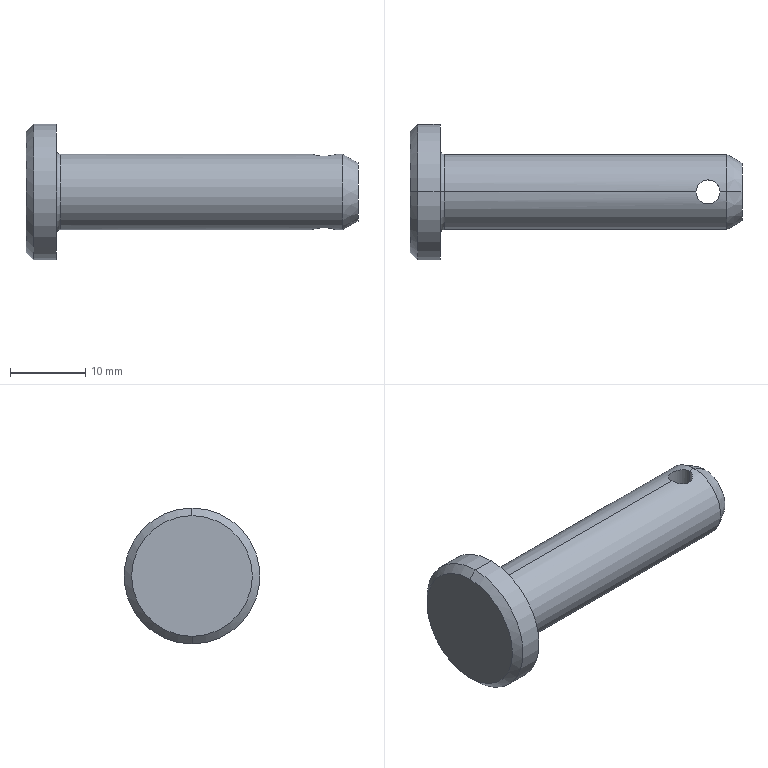Part | SolidWorks | features Chamfer 1, Fillet 1, ICE 1, Revolution 1 | 1 solid | 15 faces | box 44 x 18 x 18 mm | volume 4022 mm3 | cylinder 6 | cone 4 | plane 3 | torus 2 | commonest cylinder face diameters 3.2 x2 10 x2 18 x2
STEP:
#1=CARTESIAN_POINT('',(44.,0.,-3.845));
#2=VERTEX_POINT('',#1);
#3=CARTESIAN_POINT('',(44.,0.,3.845));
#4=VERTEX_POINT('',#3);
#5=CARTESIAN_POINT('',(44.,0.,0.));
#6=DIRECTION('',(1.,0.,0.));
#7=DIRECTION('',(0.,0.,-1.));
#8=AXIS2_PLACEMENT_3D('',#5,#6,#7);
#9=CIRCLE('',#8,3.845);
#10=EDGE_CURVE('',#2,#4,#9,.T.);
#11=ORIENTED_EDGE('',*,*,#10,.F.);
#12=CARTESIAN_POINT('',(42.,0.,-5.));
#13=VERTEX_POINT('',#12);
#14=CARTESIAN_POINT('',(44.,0.,-3.845));
#15=DIRECTION('',(-0.866,0.,-0.5));
#16=VECTOR('',#15,1000.);
#17=LINE('',#14,#16);
#18=EDGE_CURVE('',#2,#13,#17,.T.);
#19=ORIENTED_EDGE('',*,*,#18,.T.);
#20=CARTESIAN_POINT('',(42.,0.,5.));
#21=VERTEX_POINT('',#20);
#22=CARTESIAN_POINT('',(42.,0.,0.));
#23=DIRECTION('',(-1.,0.,0.));
#24=DIRECTION('',(0.,0.,-1.));
#25=AXIS2_PLACEMENT_3D('',#22,#23,#24);
#26=CIRCLE('',#25,5.);
#27=EDGE_CURVE('',#21,#13,#26,.T.);
#28=ORIENTED_EDGE('',*,*,#27,.F.);
#29=CARTESIAN_POINT('',(44.,0.,3.845));
#30=DIRECTION('',(-0.866,0.,0.5));
#31=VECTOR('',#30,1000.);
#32=LINE('',#29,#31);
#33=EDGE_CURVE('',#4,#21,#32,.T.);
#34=ORIENTED_EDGE('',*,*,#33,.F.);
#35=EDGE_LOOP('',(#11,#19,#28,#34));
#36=FACE_OUTER_BOUND('',#35,.T.);
#37=CARTESIAN_POINT('',(44.,0.,0.));
#38=DIRECTION('',(-1.,0.,0.));
#39=DIRECTION('',(0.,0.,1.));
#40=AXIS2_PLACEMENT_3D('',#37,#38,#39);
#41=CONICAL_SURFACE('',#40,3.845,0.5236);
#42=ADVANCED_FACE('',(#36),#41,.T.);
#43=CARTESIAN_POINT('',(4.6,0.,5.));
#44=VERTEX_POINT('',#43);
#45=CARTESIAN_POINT('',(4.6,0.,-5.));
#46=VERTEX_POINT('',#45);
#47=CARTESIAN_POINT('',(4.6,0.,0.));
#48=DIRECTION('',(1.,0.,0.));
#49=DIRECTION('',(0.,0.,-1.));
#50=AXIS2_PLACEMENT_3D('',#47,#48,#49);
#51=CIRCLE('',#50,5.);
#52=EDGE_CURVE('',#44,#46,#51,.T.);
#53=ORIENTED_EDGE('',*,*,#52,.F.);
#54=CARTESIAN_POINT('',(4.,0.,5.6));
#55=VERTEX_POINT('',#54);
#56=CARTESIAN_POINT('',(4.6,0.,5.6));
#57=DIRECTION('',(0.,1.,0.));
#58=DIRECTION('',(0.,0.,1.));
#59=AXIS2_PLACEMENT_3D('',#56,#57,#58);
#60=CIRCLE('',#59,0.6);
#61=EDGE_CURVE('',#44,#55,#60,.T.);
#62=ORIENTED_EDGE('',*,*,#61,.T.);
#63=CARTESIAN_POINT('',(4.,0.,-5.6));
#64=VERTEX_POINT('',#63);
#65=CARTESIAN_POINT('',(4.,0.,0.));
#66=DIRECTION('',(-1.,0.,0.));
#67=DIRECTION('',(0.,0.,-1.));
#68=AXIS2_PLACEMENT_3D('',#65,#66,#67);
#69=CIRCLE('',#68,5.6);
#70=EDGE_CURVE('',#64,#55,#69,.T.);
#71=ORIENTED_EDGE('',*,*,#70,.F.);
#72=CARTESIAN_POINT('',(4.6,0.,-5.6));
#73=DIRECTION('',(0.,-1.,0.));
#74=DIRECTION('',(0.,0.,-1.));
#75=AXIS2_PLACEMENT_3D('',#72,#73,#74);
#76=CIRCLE('',#75,0.6);
#77=EDGE_CURVE('',#46,#64,#76,.T.);
#78=ORIENTED_EDGE('',*,*,#77,.F.);
#79=EDGE_LOOP('',(#53,#62,#71,#78));
#80=FACE_OUTER_BOUND('',#79,.T.);
#81=CARTESIAN_POINT('',(4.6,0.,0.));
#82=DIRECTION('',(1.,0.,0.));
#83=DIRECTION('',(0.,0.,-1.));
#84=AXIS2_PLACEMENT_3D('',#81,#82,#83);
#85=TOROIDAL_SURFACE('',#84,5.6,0.6);
#86=ADVANCED_FACE('',(#80),#85,.F.);
#87=CARTESIAN_POINT('',(41.1,0.,-5.));
#88=VERTEX_POINT('',#87);
#89=CARTESIAN_POINT('',(37.9,0.,-5.));
#90=VERTEX_POINT('',#89);
#91=CARTESIAN_POINT('',(41.1,0.,-5.));
#92=CARTESIAN_POINT('',(41.1,-0.2097,-5.));
#93=CARTESIAN_POINT('',(41.058,-0.4215,-4.986));
#94=CARTESIAN_POINT('',(40.937,-0.711,-4.95));
#95=CARTESIAN_POINT('',(40.887,-0.8046,-4.936));
#96=CARTESIAN_POINT('',(40.771,-0.9775,-4.904));
#97=CARTESIAN_POINT('',(40.705,-1.058,-4.887));
#98=CARTESIAN_POINT('',(40.484,-1.279,-4.836));
#99=CARTESIAN_POINT('',(40.309,-1.396,-4.802));
#100=CARTESIAN_POINT('',(40.017,-1.518,-4.764));
#101=CARTESIAN_POINT('',(39.917,-1.548,-4.754));
#102=CARTESIAN_POINT('',(39.712,-1.589,-4.741));
#103=CARTESIAN_POINT('',(39.605,-1.6,-4.737));
#104=CARTESIAN_POINT('',(39.395,-1.6,-4.737));
#105=CARTESIAN_POINT('',(39.29,-1.59,-4.741));
#106=CARTESIAN_POINT('',(39.084,-1.548,-4.754));
#107=CARTESIAN_POINT('',(38.982,-1.517,-4.764));
#108=CARTESIAN_POINT('',(38.693,-1.397,-4.802));
#109=CARTESIAN_POINT('',(38.516,-1.278,-4.836));
#110=CARTESIAN_POINT('',(38.296,-1.058,-4.887));
#111=CARTESIAN_POINT('',(38.228,-0.9767,-4.904));
#112=CARTESIAN_POINT('',(38.113,-0.8036,-4.936));
#113=CARTESIAN_POINT('',(38.063,-0.7121,-4.95));
#114=CARTESIAN_POINT('',(37.983,-0.5188,-4.974));
#115=CARTESIAN_POINT('',(37.952,-0.4167,-4.984));
#116=CARTESIAN_POINT('',(37.911,-0.2111,-4.997));
#117=CARTESIAN_POINT('',(37.9,-0.1064,-5.));
#118=CARTESIAN_POINT('',(37.9,0.,-5.));
#119=B_SPLINE_CURVE_WITH_KNOTS('',3,(#91,#92,#93,#94,#95,#96,#97,#98,#99,#100,#101,#102,#103,#104,#105,#106,#107,#108,#109,#110,#111,#112,#113,#114,#115,#116,#117,#118),.UNSPECIFIED.,.F.,.F.,(4,2,2,2,2,2,2,2,2,2,2,2,2,4),(0.005036,0.005665,0.00598,0.006294,0.006924,0.007238,0.007553,0.007867,0.008182,0.008811,0.009126,0.009441,0.009755,0.01007),.UNSPECIFIED.);
#120=EDGE_CURVE('',#88,#90,#119,.T.);
#121=ORIENTED_EDGE('',*,*,#120,.T.);
#122=CARTESIAN_POINT('',(37.9,0.,5.));
#123=VERTEX_POINT('',#122);
#124=CARTESIAN_POINT('',(37.9,0.,-9.));
#125=DIRECTION('',(0.,0.,1.));
#126=VECTOR('',#125,1000.);
#127=LINE('',#124,#126);
#128=EDGE_CURVE('',#90,#123,#127,.T.);
#129=ORIENTED_EDGE('',*,*,#128,.T.);
#130=CARTESIAN_POINT('',(41.1,0.,5.));
#131=VERTEX_POINT('',#130);
#132=CARTESIAN_POINT('',(37.9,0.,5.));
#133=CARTESIAN_POINT('',(37.9,-0.2097,5.));
#134=CARTESIAN_POINT('',(37.942,-0.4215,4.986));
#135=CARTESIAN_POINT('',(38.063,-0.711,4.95));
#136=CARTESIAN_POINT('',(38.113,-0.8046,4.936));
#137=CARTESIAN_POINT('',(38.229,-0.9775,4.904));
#138=CARTESIAN_POINT('',(38.295,-1.058,4.887));
#139=CARTESIAN_POINT('',(38.516,-1.279,4.836));
#140=CARTESIAN_POINT('',(38.691,-1.396,4.802));
#141=CARTESIAN_POINT('',(38.983,-1.518,4.764));
#142=CARTESIAN_POINT('',(39.083,-1.548,4.754));
#143=CARTESIAN_POINT('',(39.288,-1.589,4.741));
#144=CARTESIAN_POINT('',(39.395,-1.6,4.737));
#145=CARTESIAN_POINT('',(39.605,-1.6,4.737));
#146=CARTESIAN_POINT('',(39.71,-1.59,4.741));
#147=CARTESIAN_POINT('',(39.916,-1.548,4.754));
#148=CARTESIAN_POINT('',(40.018,-1.517,4.764));
#149=CARTESIAN_POINT('',(40.307,-1.397,4.802));
#150=CARTESIAN_POINT('',(40.484,-1.278,4.836));
#151=CARTESIAN_POINT('',(40.704,-1.058,4.887));
#152=CARTESIAN_POINT('',(40.772,-0.9767,4.904));
#153=CARTESIAN_POINT('',(40.887,-0.8036,4.936));
#154=CARTESIAN_POINT('',(40.937,-0.7121,4.95));
#155=CARTESIAN_POINT('',(41.017,-0.5188,4.974));
#156=CARTESIAN_POINT('',(41.048,-0.4167,4.984));
#157=CARTESIAN_POINT('',(41.089,-0.2111,4.997));
#158=CARTESIAN_POINT('',(41.1,-0.1064,5.));
#159=CARTESIAN_POINT('',(41.1,0.,5.));
#160=B_SPLINE_CURVE_WITH_KNOTS('',3,(#132,#133,#134,#135,#136,#137,#138,#139,#140,#141,#142,#143,#144,#145,#146,#147,#148,#149,#150,#151,#152,#153,#154,#155,#156,#157,#158,#159),.UNSPECIFIED.,.F.,.F.,(4,2,2,2,2,2,2,2,2,2,2,2,2,4),(0.005036,0.005665,0.00598,0.006294,0.006924,0.007238,0.007553,0.007867,0.008182,0.008811,0.009126,0.009441,0.009755,0.01007),.UNSPECIFIED.);
#161=EDGE_CURVE('',#123,#131,#160,.T.);
#162=ORIENTED_EDGE('',*,*,#161,.T.);
#163=CARTESIAN_POINT('',(41.1,0.,-9.));
#164=DIRECTION('',(0.,0.,1.));
#165=VECTOR('',#164,1000.);
#166=LINE('',#163,#165);
#167=EDGE_CURVE('',#88,#131,#166,.T.);
#168=ORIENTED_EDGE('',*,*,#167,.F.);
#169=EDGE_LOOP('',(#121,#129,#162,#168));
#170=FACE_OUTER_BOUND('',#169,.T.);
#171=CARTESIAN_POINT('',(39.5,0.,-9.));
#172=DIRECTION('',(0.,0.,1.));
#173=DIRECTION('',(1.,0.,0.));
#174=AXIS2_PLACEMENT_3D('',#171,#172,#173);
#175=CYLINDRICAL_SURFACE('',#174,1.6);
#176=ADVANCED_FACE('',(#170),#175,.F.);
#177=CARTESIAN_POINT('',(4.6,0.,0.));
#178=DIRECTION('',(1.,0.,0.));
#179=DIRECTION('',(0.,0.,-1.));
#180=AXIS2_PLACEMENT_3D('',#177,#178,#179);
#181=CIRCLE('',#180,5.);
#182=EDGE_CURVE('',#46,#44,#181,.T.);
#183=ORIENTED_EDGE('',*,*,#182,.T.);
#184=CARTESIAN_POINT('',(0.,0.,5.));
#185=DIRECTION('',(1.,0.,0.));
#186=VECTOR('',#185,1000.);
#187=LINE('',#184,#186);
#188=EDGE_CURVE('',#44,#123,#187,.T.);
#189=ORIENTED_EDGE('',*,*,#188,.T.);
#190=CARTESIAN_POINT('',(41.1,0.,5.));
#191=CARTESIAN_POINT('',(41.1,0.1065,5.));
#192=CARTESIAN_POINT('',(41.089,0.211,4.997));
#193=CARTESIAN_POINT('',(41.048,0.4165,4.984));
#194=CARTESIAN_POINT('',(41.017,0.5185,4.974));
#195=CARTESIAN_POINT('',(40.937,0.712,4.95));
#196=CARTESIAN_POINT('',(40.887,0.8037,4.936));
#197=CARTESIAN_POINT('',(40.771,0.9771,4.904));
#198=CARTESIAN_POINT('',(40.704,1.059,4.887));
#199=CARTESIAN_POINT('',(40.484,1.278,4.836));
#200=CARTESIAN_POINT('',(40.307,1.397,4.802));
#201=CARTESIAN_POINT('',(40.019,1.517,4.764));
#202=CARTESIAN_POINT('',(39.917,1.548,4.754));
#203=CARTESIAN_POINT('',(39.71,1.59,4.741));
#204=CARTESIAN_POINT('',(39.606,1.6,4.737));
#205=CARTESIAN_POINT('',(39.396,1.6,4.737));
#206=CARTESIAN_POINT('',(39.289,1.589,4.741));
#207=CARTESIAN_POINT('',(39.083,1.548,4.754));
#208=CARTESIAN_POINT('',(38.983,1.518,4.764));
#209=CARTESIAN_POINT('',(38.691,1.396,4.802));
#210=CARTESIAN_POINT('',(38.516,1.278,4.836));
#211=CARTESIAN_POINT('',(38.295,1.057,4.888));
#212=CARTESIAN_POINT('',(38.229,0.9772,4.904));
#213=CARTESIAN_POINT('',(38.113,0.8043,4.936));
#214=CARTESIAN_POINT('',(38.063,0.7106,4.95));
#215=CARTESIAN_POINT('',(37.983,0.5178,4.974));
#216=CARTESIAN_POINT('',(37.952,0.418,4.984));
#217=CARTESIAN_POINT('',(37.91,0.211,4.997));
#218=CARTESIAN_POINT('',(37.9,0.1049,5.));
#219=CARTESIAN_POINT('',(37.9,0.,5.));
#220=B_SPLINE_CURVE_WITH_KNOTS('',3,(#190,#191,#192,#193,#194,#195,#196,#197,#198,#199,#200,#201,#202,#203,#204,#205,#206,#207,#208,#209,#210,#211,#212,#213,#214,#215,#216,#217,#218,#219),.UNSPECIFIED.,.F.,.F.,(4,2,2,2,2,2,2,2,2,2,2,2,2,2,4),(0.,0.0003147,0.0006295,0.0009442,0.001259,0.001888,0.002203,0.002518,0.002833,0.003147,0.003777,0.004091,0.004406,0.004721,0.005036),.UNSPECIFIED.);
#221=EDGE_CURVE('',#131,#123,#220,.T.);
#222=ORIENTED_EDGE('',*,*,#221,.F.);
#223=CARTESIAN_POINT('',(0.,0.,5.));
#224=DIRECTION('',(1.,0.,0.));
#225=VECTOR('',#224,1000.);
#226=LINE('',#223,#225);
#227=EDGE_CURVE('',#131,#21,#226,.T.);
#228=ORIENTED_EDGE('',*,*,#227,.T.);
#229=ORIENTED_EDGE('',*,*,#27,.T.);
#230=CARTESIAN_POINT('',(0.,0.,-5.));
#231=DIRECTION('',(1.,0.,0.));
#232=VECTOR('',#231,1000.);
#233=LINE('',#230,#232);
#234=EDGE_CURVE('',#88,#13,#233,.T.);
#235=ORIENTED_EDGE('',*,*,#234,.F.);
#236=CARTESIAN_POINT('',(37.9,0.,-5.));
#237=CARTESIAN_POINT('',(37.9,0.1065,-5.));
#238=CARTESIAN_POINT('',(37.911,0.211,-4.997));
#239=CARTESIAN_POINT('',(37.952,0.4165,-4.984));
#240=CARTESIAN_POINT('',(37.983,0.5185,-4.974));
#241=CARTESIAN_POINT('',(38.063,0.712,-4.95));
#242=CARTESIAN_POINT('',(38.113,0.8037,-4.936));
#243=CARTESIAN_POINT('',(38.229,0.9771,-4.904));
#244=CARTESIAN_POINT('',(38.296,1.059,-4.887));
#245=CARTESIAN_POINT('',(38.516,1.278,-4.836));
#246=CARTESIAN_POINT('',(38.693,1.397,-4.802));
#247=CARTESIAN_POINT('',(38.981,1.517,-4.764));
#248=CARTESIAN_POINT('',(39.083,1.548,-4.754));
#249=CARTESIAN_POINT('',(39.29,1.59,-4.741));
#250=CARTESIAN_POINT('',(39.394,1.6,-4.737));
#251=CARTESIAN_POINT('',(39.604,1.6,-4.737));
#252=CARTESIAN_POINT('',(39.711,1.589,-4.741));
#253=CARTESIAN_POINT('',(39.917,1.548,-4.754));
#254=CARTESIAN_POINT('',(40.017,1.518,-4.764));
#255=CARTESIAN_POINT('',(40.309,1.396,-4.802));
#256=CARTESIAN_POINT('',(40.484,1.278,-4.836));
#257=CARTESIAN_POINT('',(40.705,1.057,-4.888));
#258=CARTESIAN_POINT('',(40.771,0.9772,-4.904));
#259=CARTESIAN_POINT('',(40.887,0.8043,-4.936));
#260=CARTESIAN_POINT('',(40.937,0.7106,-4.95));
#261=CARTESIAN_POINT('',(41.017,0.5178,-4.974));
#262=CARTESIAN_POINT('',(41.048,0.418,-4.984));
#263=CARTESIAN_POINT('',(41.09,0.211,-4.997));
#264=CARTESIAN_POINT('',(41.1,0.1049,-5.));
#265=CARTESIAN_POINT('',(41.1,0.,-5.));
#266=B_SPLINE_CURVE_WITH_KNOTS('',3,(#236,#237,#238,#239,#240,#241,#242,#243,#244,#245,#246,#247,#248,#249,#250,#251,#252,#253,#254,#255,#256,#257,#258,#259,#260,#261,#262,#263,#264,#265),.UNSPECIFIED.,.F.,.F.,(4,2,2,2,2,2,2,2,2,2,2,2,2,2,4),(0.,0.0003147,0.0006295,0.0009442,0.001259,0.001888,0.002203,0.002518,0.002833,0.003147,0.003777,0.004091,0.004406,0.004721,0.005036),.UNSPECIFIED.);
#267=EDGE_CURVE('',#90,#88,#266,.T.);
#268=ORIENTED_EDGE('',*,*,#267,.F.);
#269=CARTESIAN_POINT('',(0.,0.,-5.));
#270=DIRECTION('',(1.,0.,0.));
#271=VECTOR('',#270,1000.);
#272=LINE('',#269,#271);
#273=EDGE_CURVE('',#46,#90,#272,.T.);
#274=ORIENTED_EDGE('',*,*,#273,.F.);
#275=EDGE_LOOP('',(#183,#189,#222,#228,#229,#235,#268,#274));
#276=FACE_OUTER_BOUND('',#275,.T.);
#277=CARTESIAN_POINT('',(0.,0.,0.));
#278=DIRECTION('',(1.,0.,0.));
#279=DIRECTION('',(0.,0.,-1.));
#280=AXIS2_PLACEMENT_3D('',#277,#278,#279);
#281=CYLINDRICAL_SURFACE('',#280,5.);
#282=ADVANCED_FACE('',(#276),#281,.T.);
#283=CARTESIAN_POINT('',(1.,0.,-9.));
#284=VERTEX_POINT('',#283);
#285=CARTESIAN_POINT('',(1.,0.,9.));
#286=VERTEX_POINT('',#285);
#287=CARTESIAN_POINT('',(1.,0.,0.));
#288=DIRECTION('',(1.,0.,0.));
#289=DIRECTION('',(0.,0.,-1.));
#290=AXIS2_PLACEMENT_3D('',#287,#288,#289);
#291=CIRCLE('',#290,9.);
#292=EDGE_CURVE('',#284,#286,#291,.T.);
#293=ORIENTED_EDGE('',*,*,#292,.T.);
#294=CARTESIAN_POINT('',(4.,0.,9.));
#295=VERTEX_POINT('',#294);
#296=CARTESIAN_POINT('',(0.,0.,9.));
#297=DIRECTION('',(1.,0.,0.));
#298=VECTOR('',#297,1000.);
#299=LINE('',#296,#298);
#300=EDGE_CURVE('',#286,#295,#299,.T.);
#301=ORIENTED_EDGE('',*,*,#300,.T.);
#302=CARTESIAN_POINT('',(4.,0.,-9.));
#303=VERTEX_POINT('',#302);
#304=CARTESIAN_POINT('',(4.,0.,0.));
#305=DIRECTION('',(1.,0.,0.));
#306=DIRECTION('',(0.,0.,-1.));
#307=AXIS2_PLACEMENT_3D('',#304,#305,#306);
#308=CIRCLE('',#307,9.);
#309=EDGE_CURVE('',#303,#295,#308,.T.);
#310=ORIENTED_EDGE('',*,*,#309,.F.);
#311=CARTESIAN_POINT('',(0.,0.,-9.));
#312=DIRECTION('',(1.,0.,0.));
#313=VECTOR('',#312,1000.);
#314=LINE('',#311,#313);
#315=EDGE_CURVE('',#284,#303,#314,.T.);
#316=ORIENTED_EDGE('',*,*,#315,.F.);
#317=EDGE_LOOP('',(#293,#301,#310,#316));
#318=FACE_OUTER_BOUND('',#317,.T.);
#319=CARTESIAN_POINT('',(0.,0.,0.));
#320=DIRECTION('',(1.,0.,0.));
#321=DIRECTION('',(0.,0.,-1.));
#322=AXIS2_PLACEMENT_3D('',#319,#320,#321);
#323=CYLINDRICAL_SURFACE('',#322,9.);
#324=ADVANCED_FACE('',(#318),#323,.T.);
#325=CARTESIAN_POINT('',(0.,0.,-8.));
#326=VERTEX_POINT('',#325);
#327=CARTESIAN_POINT('',(0.,0.,8.));
#328=VERTEX_POINT('',#327);
#329=CARTESIAN_POINT('',(0.,0.,0.));
#330=DIRECTION('',(1.,0.,0.));
#331=DIRECTION('',(0.,0.,-1.));
#332=AXIS2_PLACEMENT_3D('',#329,#330,#331);
#333=CIRCLE('',#332,8.);
#334=EDGE_CURVE('',#326,#328,#333,.T.);
#335=ORIENTED_EDGE('',*,*,#334,.T.);
#336=CARTESIAN_POINT('',(1.,0.,9.));
#337=DIRECTION('',(0.7071,0.,0.7071));
#338=VECTOR('',#337,1000.);
#339=LINE('',#336,#338);
#340=EDGE_CURVE('',#328,#286,#339,.T.);
#341=ORIENTED_EDGE('',*,*,#340,.T.);
#342=ORIENTED_EDGE('',*,*,#292,.F.);
#343=CARTESIAN_POINT('',(1.,0.,-9.));
#344=DIRECTION('',(0.7071,0.,-0.7071));
#345=VECTOR('',#344,1000.);
#346=LINE('',#343,#345);
#347=EDGE_CURVE('',#326,#284,#346,.T.);
#348=ORIENTED_EDGE('',*,*,#347,.F.);
#349=EDGE_LOOP('',(#335,#341,#342,#348));
#350=FACE_OUTER_BOUND('',#349,.T.);
#351=CARTESIAN_POINT('',(1.,0.,0.));
#352=DIRECTION('',(1.,0.,0.));
#353=DIRECTION('',(0.,0.,-1.));
#354=AXIS2_PLACEMENT_3D('',#351,#352,#353);
#355=CONICAL_SURFACE('',#354,9.,0.7854);
#356=ADVANCED_FACE('',(#350),#355,.T.);
#357=ORIENTED_EDGE('',*,*,#334,.F.);
#358=CARTESIAN_POINT('',(0.,0.,0.));
#359=DIRECTION('',(1.,0.,0.));
#360=DIRECTION('',(0.,0.,-1.));
#361=AXIS2_PLACEMENT_3D('',#358,#359,#360);
#362=CIRCLE('',#361,8.);
#363=EDGE_CURVE('',#328,#326,#362,.T.);
#364=ORIENTED_EDGE('',*,*,#363,.F.);
#365=EDGE_LOOP('',(#357,#364));
#366=FACE_OUTER_BOUND('',#365,.T.);
#367=CARTESIAN_POINT('',(0.,0.,0.));
#368=DIRECTION('',(-1.,0.,0.));
#369=DIRECTION('',(0.,0.,1.));
#370=AXIS2_PLACEMENT_3D('',#367,#368,#369);
#371=PLANE('',#370);
#372=ADVANCED_FACE('',(#366),#371,.T.);
#373=ORIENTED_EDGE('',*,*,#340,.F.);
#374=ORIENTED_EDGE('',*,*,#363,.T.);
#375=ORIENTED_EDGE('',*,*,#347,.T.);
#376=CARTESIAN_POINT('',(1.,0.,0.));
#377=DIRECTION('',(1.,0.,0.));
#378=DIRECTION('',(0.,0.,-1.));
#379=AXIS2_PLACEMENT_3D('',#376,#377,#378);
#380=CIRCLE('',#379,9.);
#381=EDGE_CURVE('',#286,#284,#380,.T.);
#382=ORIENTED_EDGE('',*,*,#381,.F.);
#383=EDGE_LOOP('',(#373,#374,#375,#382));
#384=FACE_OUTER_BOUND('',#383,.T.);
#385=CARTESIAN_POINT('',(1.,0.,0.));
#386=DIRECTION('',(1.,0.,0.));
#387=DIRECTION('',(0.,0.,-1.));
#388=AXIS2_PLACEMENT_3D('',#385,#386,#387);
#389=CONICAL_SURFACE('',#388,9.,0.7854);
#390=ADVANCED_FACE('',(#384),#389,.T.);
#391=ORIENTED_EDGE('',*,*,#300,.F.);
#392=ORIENTED_EDGE('',*,*,#381,.T.);
#393=ORIENTED_EDGE('',*,*,#315,.T.);
#394=CARTESIAN_POINT('',(4.,0.,0.));
#395=DIRECTION('',(1.,0.,0.));
#396=DIRECTION('',(0.,0.,-1.));
#397=AXIS2_PLACEMENT_3D('',#394,#395,#396);
#398=CIRCLE('',#397,9.);
#399=EDGE_CURVE('',#295,#303,#398,.T.);
#400=ORIENTED_EDGE('',*,*,#399,.F.);
#401=EDGE_LOOP('',(#391,#392,#393,#400));
#402=FACE_OUTER_BOUND('',#401,.T.);
#403=CARTESIAN_POINT('',(0.,0.,0.));
#404=DIRECTION('',(1.,0.,0.));
#405=DIRECTION('',(0.,0.,-1.));
#406=AXIS2_PLACEMENT_3D('',#403,#404,#405);
#407=CYLINDRICAL_SURFACE('',#406,9.);
#408=ADVANCED_FACE('',(#402),#407,.T.);
#409=ORIENTED_EDGE('',*,*,#70,.T.);
#410=CARTESIAN_POINT('',(4.,0.,0.));
#411=DIRECTION('',(-1.,0.,0.));
#412=DIRECTION('',(0.,0.,-1.));
#413=AXIS2_PLACEMENT_3D('',#410,#411,#412);
#414=CIRCLE('',#413,5.6);
#415=EDGE_CURVE('',#55,#64,#414,.T.);
#416=ORIENTED_EDGE('',*,*,#415,.T.);
#417=EDGE_LOOP('',(#409,#416));
#418=FACE_BOUND('',#417,.T.);
#419=ORIENTED_EDGE('',*,*,#309,.T.);
#420=ORIENTED_EDGE('',*,*,#399,.T.);
#421=EDGE_LOOP('',(#419,#420));
#422=FACE_OUTER_BOUND('',#421,.T.);
#423=CARTESIAN_POINT('',(4.,9.,0.));
#424=DIRECTION('',(1.,0.,0.));
#425=DIRECTION('',(0.,0.,-1.));
#426=AXIS2_PLACEMENT_3D('',#423,#424,#425);
#427=PLANE('',#426);
#428=ADVANCED_FACE('',(#418,#422),#427,.T.);
#429=ORIENTED_EDGE('',*,*,#188,.F.);
#430=ORIENTED_EDGE('',*,*,#52,.T.);
#431=ORIENTED_EDGE('',*,*,#273,.T.);
#432=ORIENTED_EDGE('',*,*,#120,.F.);
#433=ORIENTED_EDGE('',*,*,#234,.T.);
#434=CARTESIAN_POINT('',(42.,0.,0.));
#435=DIRECTION('',(-1.,0.,0.));
#436=DIRECTION('',(0.,0.,-1.));
#437=AXIS2_PLACEMENT_3D('',#434,#435,#436);
#438=CIRCLE('',#437,5.);
#439=EDGE_CURVE('',#13,#21,#438,.T.);
#440=ORIENTED_EDGE('',*,*,#439,.T.);
#441=ORIENTED_EDGE('',*,*,#227,.F.);
#442=ORIENTED_EDGE('',*,*,#161,.F.);
#443=EDGE_LOOP('',(#429,#430,#431,#432,#433,#440,#441,#442));
#444=FACE_OUTER_BOUND('',#443,.T.);
#445=CARTESIAN_POINT('',(0.,0.,0.));
#446=DIRECTION('',(1.,0.,0.));
#447=DIRECTION('',(0.,0.,-1.));
#448=AXIS2_PLACEMENT_3D('',#445,#446,#447);
#449=CYLINDRICAL_SURFACE('',#448,5.);
#450=ADVANCED_FACE('',(#444),#449,.T.);
#451=CARTESIAN_POINT('',(44.,0.,0.));
#452=DIRECTION('',(1.,0.,0.));
#453=DIRECTION('',(0.,0.,-1.));
#454=AXIS2_PLACEMENT_3D('',#451,#452,#453);
#455=CIRCLE('',#454,3.845);
#456=EDGE_CURVE('',#4,#2,#455,.T.);
#457=ORIENTED_EDGE('',*,*,#456,.T.);
#458=ORIENTED_EDGE('',*,*,#10,.T.);
#459=EDGE_LOOP('',(#457,#458));
#460=FACE_OUTER_BOUND('',#459,.T.);
#461=CARTESIAN_POINT('',(44.,5.,0.));
#462=DIRECTION('',(1.,0.,0.));
#463=DIRECTION('',(0.,0.,-1.));
#464=AXIS2_PLACEMENT_3D('',#461,#462,#463);
#465=PLANE('',#464);
#466=ADVANCED_FACE('',(#460),#465,.T.);
#467=ORIENTED_EDGE('',*,*,#128,.F.);
#468=ORIENTED_EDGE('',*,*,#267,.T.);
#469=ORIENTED_EDGE('',*,*,#167,.T.);
#470=ORIENTED_EDGE('',*,*,#221,.T.);
#471=EDGE_LOOP('',(#467,#468,#469,#470));
#472=FACE_OUTER_BOUND('',#471,.T.);
#473=CARTESIAN_POINT('',(39.5,0.,-9.));
#474=DIRECTION('',(0.,0.,1.));
#475=DIRECTION('',(1.,0.,0.));
#476=AXIS2_PLACEMENT_3D('',#473,#474,#475);
#477=CYLINDRICAL_SURFACE('',#476,1.6);
#478=ADVANCED_FACE('',(#472),#477,.F.);
#479=ORIENTED_EDGE('',*,*,#61,.F.);
#480=ORIENTED_EDGE('',*,*,#182,.F.);
#481=ORIENTED_EDGE('',*,*,#77,.T.);
#482=ORIENTED_EDGE('',*,*,#415,.F.);
#483=EDGE_LOOP('',(#479,#480,#481,#482));
#484=FACE_OUTER_BOUND('',#483,.T.);
#485=CARTESIAN_POINT('',(4.6,0.,0.));
#486=DIRECTION('',(1.,0.,0.));
#487=DIRECTION('',(0.,0.,-1.));
#488=AXIS2_PLACEMENT_3D('',#485,#486,#487);
#489=TOROIDAL_SURFACE('',#488,5.6,0.6);
#490=ADVANCED_FACE('',(#484),#489,.F.);
#491=ORIENTED_EDGE('',*,*,#18,.F.);
#492=ORIENTED_EDGE('',*,*,#456,.F.);
#493=ORIENTED_EDGE('',*,*,#33,.T.);
#494=ORIENTED_EDGE('',*,*,#439,.F.);
#495=EDGE_LOOP('',(#491,#492,#493,#494));
#496=FACE_OUTER_BOUND('',#495,.T.);
#497=CARTESIAN_POINT('',(44.,0.,0.));
#498=DIRECTION('',(-1.,0.,0.));
#499=DIRECTION('',(0.,0.,1.));
#500=AXIS2_PLACEMENT_3D('',#497,#498,#499);
#501=CONICAL_SURFACE('',#500,3.845,0.5236);
#502=ADVANCED_FACE('',(#496),#501,.T.);
#503=CLOSED_SHELL('',(#42,#86,#176,#282,#324,#356,#372,#390,#408,#428,#450,#466,#478,#490,#502));
#504=MANIFOLD_SOLID_BREP('',#503);
#505=CARTESIAN_POINT('',(0.,0.,0.));
#506=DIRECTION('',(0.,0.,1.));
#507=DIRECTION('',(1.,0.,0.));
#508=AXIS2_PLACEMENT_3D('',#505,#506,#507);
#509=(LENGTH_UNIT()NAMED_UNIT(*)SI_UNIT(.MILLI.,.METRE.));
#510=UNCERTAINTY_MEASURE_WITH_UNIT(LENGTH_MEASURE(0.00001),#509,'','');
#511=(NAMED_UNIT(*)PLANE_ANGLE_UNIT()SI_UNIT($,.RADIAN.));
#512=(NAMED_UNIT(*)SI_UNIT($,.STERADIAN.)SOLID_ANGLE_UNIT());
#513=(GEOMETRIC_REPRESENTATION_CONTEXT(3)GLOBAL_UNCERTAINTY_ASSIGNED_CONTEXT((#510))GLOBAL_UNIT_ASSIGNED_CONTEXT((#509,#511,#512))REPRESENTATION_CONTEXT('',''));
#514=ADVANCED_BREP_SHAPE_REPRESENTATION('',(#504,#508),#513);